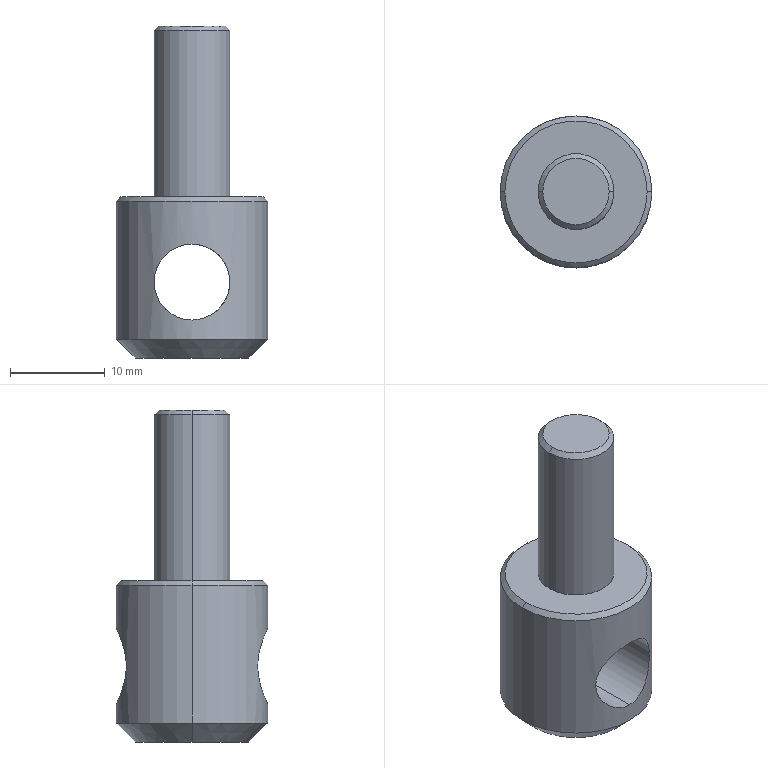Part | NX | features BREP 1 | 1 solid | 15 faces | box 16 x 16 x 35 mm | volume 3443 mm3 | cone 6 | cylinder 6 | plane 3 | commonest cylinder face diameters 8 x4 16 x2
STEP:
#1=CARTESIAN_POINT('',(-1.629,-43.754,35.));
#2=VERTEX_POINT('',#1);
#3=CARTESIAN_POINT('',(-8.629,-43.754,35.));
#4=VERTEX_POINT('',#3);
#5=CARTESIAN_POINT('',(-5.129,-43.754,35.));
#6=DIRECTION('',(0.,0.,1.));
#7=DIRECTION('',(1.,0.,0.));
#8=AXIS2_PLACEMENT_3D('',#5,#6,#7);
#9=CIRCLE('',#8,3.5);
#10=EDGE_CURVE('',#2,#4,#9,.T.);
#11=ORIENTED_EDGE('',*,*,#10,.F.);
#12=CARTESIAN_POINT('',(-1.129,-43.754,34.5));
#13=VERTEX_POINT('',#12);
#14=CARTESIAN_POINT('',(-1.629,-43.754,35.));
#15=DIRECTION('',(0.7071,0.,-0.7071));
#16=VECTOR('',#15,1000.);
#17=LINE('',#14,#16);
#18=EDGE_CURVE('',#2,#13,#17,.T.);
#19=ORIENTED_EDGE('',*,*,#18,.T.);
#20=CARTESIAN_POINT('',(-9.129,-43.754,34.5));
#21=VERTEX_POINT('',#20);
#22=CARTESIAN_POINT('',(-5.129,-43.754,34.5));
#23=DIRECTION('',(0.,0.,-1.));
#24=DIRECTION('',(1.,0.,0.));
#25=AXIS2_PLACEMENT_3D('',#22,#23,#24);
#26=CIRCLE('',#25,4.);
#27=EDGE_CURVE('',#21,#13,#26,.T.);
#28=ORIENTED_EDGE('',*,*,#27,.F.);
#29=CARTESIAN_POINT('',(-8.629,-43.754,35.));
#30=DIRECTION('',(-0.7071,0.,-0.7071));
#31=VECTOR('',#30,1000.);
#32=LINE('',#29,#31);
#33=EDGE_CURVE('',#4,#21,#32,.T.);
#34=ORIENTED_EDGE('',*,*,#33,.F.);
#35=EDGE_LOOP('',(#11,#19,#28,#34));
#36=FACE_BOUND('',#35,.T.);
#37=CARTESIAN_POINT('',(-5.129,-43.754,35.));
#38=DIRECTION('',(0.,0.,-1.));
#39=DIRECTION('',(-1.,0.,0.));
#40=AXIS2_PLACEMENT_3D('',#37,#38,#39);
#41=CONICAL_SURFACE('',#40,3.5,0.7854);
#42=ADVANCED_FACE('',(#36),#41,.T.);
#43=CARTESIAN_POINT('',(2.371,-43.754,17.));
#44=VERTEX_POINT('',#43);
#45=CARTESIAN_POINT('',(-12.629,-43.754,17.));
#46=VERTEX_POINT('',#45);
#47=CARTESIAN_POINT('',(-5.129,-43.754,17.));
#48=DIRECTION('',(0.,0.,1.));
#49=DIRECTION('',(1.,0.,0.));
#50=AXIS2_PLACEMENT_3D('',#47,#48,#49);
#51=CIRCLE('',#50,7.5);
#52=EDGE_CURVE('',#44,#46,#51,.T.);
#53=ORIENTED_EDGE('',*,*,#52,.F.);
#54=CARTESIAN_POINT('',(2.871,-43.754,16.5));
#55=VERTEX_POINT('',#54);
#56=CARTESIAN_POINT('',(2.371,-43.754,17.));
#57=DIRECTION('',(0.7071,0.,-0.7071));
#58=VECTOR('',#57,1000.);
#59=LINE('',#56,#58);
#60=EDGE_CURVE('',#44,#55,#59,.T.);
#61=ORIENTED_EDGE('',*,*,#60,.T.);
#62=CARTESIAN_POINT('',(-13.129,-43.754,16.5));
#63=VERTEX_POINT('',#62);
#64=CARTESIAN_POINT('',(-5.129,-43.754,16.5));
#65=DIRECTION('',(0.,0.,-1.));
#66=DIRECTION('',(1.,0.,0.));
#67=AXIS2_PLACEMENT_3D('',#64,#65,#66);
#68=CIRCLE('',#67,8.);
#69=EDGE_CURVE('',#63,#55,#68,.T.);
#70=ORIENTED_EDGE('',*,*,#69,.F.);
#71=CARTESIAN_POINT('',(-12.629,-43.754,17.));
#72=DIRECTION('',(-0.7071,0.,-0.7071));
#73=VECTOR('',#72,1000.);
#74=LINE('',#71,#73);
#75=EDGE_CURVE('',#46,#63,#74,.T.);
#76=ORIENTED_EDGE('',*,*,#75,.F.);
#77=EDGE_LOOP('',(#53,#61,#70,#76));
#78=FACE_BOUND('',#77,.T.);
#79=CARTESIAN_POINT('',(-5.129,-43.754,17.));
#80=DIRECTION('',(0.,0.,-1.));
#81=DIRECTION('',(-1.,0.,0.));
#82=AXIS2_PLACEMENT_3D('',#79,#80,#81);
#83=CONICAL_SURFACE('',#82,7.5,0.7854);
#84=ADVANCED_FACE('',(#78),#83,.T.);
#85=ORIENTED_EDGE('',*,*,#27,.T.);
#86=CARTESIAN_POINT('',(-1.129,-43.754,17.));
#87=VERTEX_POINT('',#86);
#88=CARTESIAN_POINT('',(-1.129,-43.754,35.));
#89=DIRECTION('',(0.,0.,-1.));
#90=VECTOR('',#89,1000.);
#91=LINE('',#88,#90);
#92=EDGE_CURVE('',#13,#87,#91,.T.);
#93=ORIENTED_EDGE('',*,*,#92,.T.);
#94=CARTESIAN_POINT('',(-9.129,-43.754,17.));
#95=VERTEX_POINT('',#94);
#96=CARTESIAN_POINT('',(-5.129,-43.754,17.));
#97=DIRECTION('',(0.,0.,1.));
#98=DIRECTION('',(1.,0.,0.));
#99=AXIS2_PLACEMENT_3D('',#96,#97,#98);
#100=CIRCLE('',#99,4.);
#101=EDGE_CURVE('',#87,#95,#100,.T.);
#102=ORIENTED_EDGE('',*,*,#101,.T.);
#103=CARTESIAN_POINT('',(-9.129,-43.754,35.));
#104=DIRECTION('',(0.,0.,-1.));
#105=VECTOR('',#104,1000.);
#106=LINE('',#103,#105);
#107=EDGE_CURVE('',#21,#95,#106,.T.);
#108=ORIENTED_EDGE('',*,*,#107,.F.);
#109=EDGE_LOOP('',(#85,#93,#102,#108));
#110=FACE_BOUND('',#109,.T.);
#111=CARTESIAN_POINT('',(-5.129,-43.754,35.));
#112=DIRECTION('',(0.,0.,-1.));
#113=DIRECTION('',(-1.,0.,0.));
#114=AXIS2_PLACEMENT_3D('',#111,#112,#113);
#115=CYLINDRICAL_SURFACE('',#114,4.);
#116=ADVANCED_FACE('',(#110),#115,.T.);
#117=CARTESIAN_POINT('',(-11.129,-43.754,0.));
#118=VERTEX_POINT('',#117);
#119=CARTESIAN_POINT('',(0.871,-43.754,0.));
#120=VERTEX_POINT('',#119);
#121=CARTESIAN_POINT('',(-5.129,-43.754,0.));
#122=DIRECTION('',(0.,0.,-1.));
#123=DIRECTION('',(1.,0.,0.));
#124=AXIS2_PLACEMENT_3D('',#121,#122,#123);
#125=CIRCLE('',#124,6.);
#126=EDGE_CURVE('',#118,#120,#125,.T.);
#127=ORIENTED_EDGE('',*,*,#126,.F.);
#128=CARTESIAN_POINT('',(-13.129,-43.754,2.));
#129=VERTEX_POINT('',#128);
#130=CARTESIAN_POINT('',(-13.129,-43.754,2.));
#131=DIRECTION('',(-0.7071,0.,0.7071));
#132=VECTOR('',#131,1000.);
#133=LINE('',#130,#132);
#134=EDGE_CURVE('',#129,#118,#133,.F.);
#135=ORIENTED_EDGE('',*,*,#134,.F.);
#136=CARTESIAN_POINT('',(2.871,-43.754,2.));
#137=VERTEX_POINT('',#136);
#138=CARTESIAN_POINT('',(-5.129,-43.754,2.));
#139=DIRECTION('',(0.,0.,1.));
#140=DIRECTION('',(1.,0.,0.));
#141=AXIS2_PLACEMENT_3D('',#138,#139,#140);
#142=CIRCLE('',#141,8.);
#143=EDGE_CURVE('',#137,#129,#142,.T.);
#144=ORIENTED_EDGE('',*,*,#143,.F.);
#145=CARTESIAN_POINT('',(2.871,-43.754,2.));
#146=DIRECTION('',(0.7071,0.,0.7071));
#147=VECTOR('',#146,1000.);
#148=LINE('',#145,#147);
#149=EDGE_CURVE('',#137,#120,#148,.F.);
#150=ORIENTED_EDGE('',*,*,#149,.T.);
#151=EDGE_LOOP('',(#127,#135,#144,#150));
#152=FACE_BOUND('',#151,.T.);
#153=CARTESIAN_POINT('',(-5.129,-43.754,2.));
#154=DIRECTION('',(0.,0.,1.));
#155=DIRECTION('',(1.,0.,0.));
#156=AXIS2_PLACEMENT_3D('',#153,#154,#155);
#157=CONICAL_SURFACE('',#156,8.,0.7854);
#158=ADVANCED_FACE('',(#152),#157,.T.);
#159=CARTESIAN_POINT('',(-5.129,-35.754,4.));
#160=VERTEX_POINT('',#159);
#161=CARTESIAN_POINT('',(-5.129,-35.754,12.));
#162=VERTEX_POINT('',#161);
#163=CARTESIAN_POINT('',(-5.129,-35.754,4.));
#164=CARTESIAN_POINT('',(-5.382,-35.754,4.));
#165=CARTESIAN_POINT('',(-5.888,-35.776,4.042));
#166=CARTESIAN_POINT('',(-6.584,-35.881,4.26));
#167=CARTESIAN_POINT('',(-7.004,-35.974,4.459));
#168=CARTESIAN_POINT('',(-7.389,-36.077,4.692));
#169=CARTESIAN_POINT('',(-7.623,-36.151,4.868));
#170=CARTESIAN_POINT('',(-7.953,-36.265,5.147));
#171=CARTESIAN_POINT('',(-8.331,-36.42,5.593));
#172=CARTESIAN_POINT('',(-8.423,-36.463,5.723));
#173=CARTESIAN_POINT('',(-8.683,-36.585,6.146));
#174=CARTESIAN_POINT('',(-8.864,-36.678,6.541));
#175=CARTESIAN_POINT('',(-9.082,-36.797,7.212));
#176=CARTESIAN_POINT('',(-9.153,-36.84,7.994));
#177=CARTESIAN_POINT('',(-9.082,-36.797,8.79));
#178=CARTESIAN_POINT('',(-8.864,-36.679,9.458));
#179=CARTESIAN_POINT('',(-8.683,-36.585,9.855));
#180=CARTESIAN_POINT('',(-8.421,-36.462,10.28));
#181=CARTESIAN_POINT('',(-8.331,-36.42,10.408));
#182=CARTESIAN_POINT('',(-7.949,-36.263,10.857));
#183=CARTESIAN_POINT('',(-7.621,-36.151,11.133));
#184=CARTESIAN_POINT('',(-7.386,-36.076,11.31));
#185=CARTESIAN_POINT('',(-7.002,-35.973,11.542));
#186=CARTESIAN_POINT('',(-6.581,-35.881,11.741));
#187=CARTESIAN_POINT('',(-5.887,-35.776,11.958));
#188=CARTESIAN_POINT('',(-5.381,-35.754,12.));
#189=CARTESIAN_POINT('',(-5.129,-35.754,12.));
#190=B_SPLINE_CURVE_WITH_KNOTS('',3,(#163,#164,#165,#166,#167,#168,#169,#170,#171,#172,#173,#174,#175,#176,#177,#178,#179,#180,#181,#182,#183,#184,#185,#186,#187,#188,#189),.UNSPECIFIED.,.F.,.F.,(4,1,1,1,1,1,1,1,1,1,1,1,1,1,1,1,1,1,1,1,1,1,1,1,4),(0.,0.0625,0.125,0.1562,0.1875,0.2188,0.25,0.2812,0.3125,0.3438,0.375,0.4375,0.5,0.5625,0.625,0.6562,0.6875,0.7188,0.75,0.7812,0.8125,0.8438,0.875,0.9375,1.),.UNSPECIFIED.);
#191=EDGE_CURVE('',#160,#162,#190,.T.);
#192=ORIENTED_EDGE('',*,*,#191,.T.);
#193=CARTESIAN_POINT('',(-5.129,-51.754,12.));
#194=VERTEX_POINT('',#193);
#195=CARTESIAN_POINT('',(-5.129,20.,12.));
#196=DIRECTION('',(0.,-1.,0.));
#197=VECTOR('',#196,1000.);
#198=LINE('',#195,#197);
#199=EDGE_CURVE('',#162,#194,#198,.T.);
#200=ORIENTED_EDGE('',*,*,#199,.T.);
#201=CARTESIAN_POINT('',(-5.129,-51.754,4.));
#202=VERTEX_POINT('',#201);
#203=CARTESIAN_POINT('',(-5.129,-51.754,12.));
#204=CARTESIAN_POINT('',(-5.382,-51.754,12.));
#205=CARTESIAN_POINT('',(-5.888,-51.731,11.958));
#206=CARTESIAN_POINT('',(-6.583,-51.626,11.74));
#207=CARTESIAN_POINT('',(-7.004,-51.534,11.541));
#208=CARTESIAN_POINT('',(-7.389,-51.43,11.308));
#209=CARTESIAN_POINT('',(-7.623,-51.356,11.132));
#210=CARTESIAN_POINT('',(-7.954,-51.242,10.852));
#211=CARTESIAN_POINT('',(-8.33,-51.088,10.409));
#212=CARTESIAN_POINT('',(-8.421,-51.045,10.279));
#213=CARTESIAN_POINT('',(-8.683,-50.923,9.855));
#214=CARTESIAN_POINT('',(-8.865,-50.829,9.457));
#215=CARTESIAN_POINT('',(-9.08,-50.711,8.796));
#216=CARTESIAN_POINT('',(-9.153,-50.668,8.005));
#217=CARTESIAN_POINT('',(-9.082,-50.71,7.212));
#218=CARTESIAN_POINT('',(-8.866,-50.828,6.547));
#219=CARTESIAN_POINT('',(-8.684,-50.922,6.148));
#220=CARTESIAN_POINT('',(-8.422,-51.045,5.722));
#221=CARTESIAN_POINT('',(-8.331,-51.087,5.593));
#222=CARTESIAN_POINT('',(-7.951,-51.243,5.146));
#223=CARTESIAN_POINT('',(-7.624,-51.356,4.869));
#224=CARTESIAN_POINT('',(-7.391,-51.43,4.694));
#225=CARTESIAN_POINT('',(-7.005,-51.533,4.459));
#226=CARTESIAN_POINT('',(-6.584,-51.626,4.26));
#227=CARTESIAN_POINT('',(-5.889,-51.731,4.042));
#228=CARTESIAN_POINT('',(-5.382,-51.754,4.));
#229=CARTESIAN_POINT('',(-5.129,-51.754,4.));
#230=B_SPLINE_CURVE_WITH_KNOTS('',3,(#203,#204,#205,#206,#207,#208,#209,#210,#211,#212,#213,#214,#215,#216,#217,#218,#219,#220,#221,#222,#223,#224,#225,#226,#227,#228,#229),.UNSPECIFIED.,.F.,.F.,(4,1,1,1,1,1,1,1,1,1,1,1,1,1,1,1,1,1,1,1,1,1,1,1,4),(0.,0.0625,0.125,0.1562,0.1875,0.2188,0.25,0.2812,0.3125,0.3438,0.375,0.4375,0.5,0.5625,0.625,0.6562,0.6875,0.7188,0.75,0.7812,0.8125,0.8438,0.875,0.9375,1.),.UNSPECIFIED.);
#231=EDGE_CURVE('',#194,#202,#230,.T.);
#232=ORIENTED_EDGE('',*,*,#231,.T.);
#233=CARTESIAN_POINT('',(-5.129,20.,4.));
#234=DIRECTION('',(0.,-1.,0.));
#235=VECTOR('',#234,1000.);
#236=LINE('',#233,#235);
#237=EDGE_CURVE('',#160,#202,#236,.T.);
#238=ORIENTED_EDGE('',*,*,#237,.F.);
#239=EDGE_LOOP('',(#192,#200,#232,#238));
#240=FACE_BOUND('',#239,.T.);
#241=CARTESIAN_POINT('',(-5.129,20.,8.));
#242=DIRECTION('',(0.,-1.,0.));
#243=DIRECTION('',(0.,0.,-1.));
#244=AXIS2_PLACEMENT_3D('',#241,#242,#243);
#245=CYLINDRICAL_SURFACE('',#244,4.);
#246=ADVANCED_FACE('',(#240),#245,.F.);
#247=ORIENTED_EDGE('',*,*,#69,.T.);
#248=CARTESIAN_POINT('',(2.871,-43.754,17.));
#249=DIRECTION('',(0.,0.,-1.));
#250=VECTOR('',#249,1000.);
#251=LINE('',#248,#250);
#252=EDGE_CURVE('',#55,#137,#251,.T.);
#253=ORIENTED_EDGE('',*,*,#252,.T.);
#254=ORIENTED_EDGE('',*,*,#143,.T.);
#255=CARTESIAN_POINT('',(-13.129,-43.754,17.));
#256=DIRECTION('',(0.,0.,-1.));
#257=VECTOR('',#256,1000.);
#258=LINE('',#255,#257);
#259=EDGE_CURVE('',#63,#129,#258,.T.);
#260=ORIENTED_EDGE('',*,*,#259,.F.);
#261=EDGE_LOOP('',(#247,#253,#254,#260));
#262=FACE_BOUND('',#261,.T.);
#263=ORIENTED_EDGE('',*,*,#191,.F.);
#264=CARTESIAN_POINT('',(-5.129,-35.754,4.));
#265=CARTESIAN_POINT('',(-4.06,-35.754,4.));
#266=CARTESIAN_POINT('',(-2.001,-36.253,4.868));
#267=CARTESIAN_POINT('',(-0.6936,-37.112,8.008));
#268=CARTESIAN_POINT('',(-1.998,-36.254,11.125));
#269=CARTESIAN_POINT('',(-4.061,-35.754,12.));
#270=CARTESIAN_POINT('',(-5.129,-35.754,12.));
#271=B_SPLINE_CURVE_WITH_KNOTS('',3,(#264,#265,#266,#267,#268,#269,#270),.UNSPECIFIED.,.F.,.F.,(4,1,1,1,4),(0.,0.25,0.5,0.75,1.),.UNSPECIFIED.);
#272=EDGE_CURVE('',#162,#160,#271,.F.);
#273=ORIENTED_EDGE('',*,*,#272,.F.);
#274=EDGE_LOOP('',(#263,#273));
#275=FACE_BOUND('',#274,.T.);
#276=CARTESIAN_POINT('',(-5.129,-43.754,17.));
#277=DIRECTION('',(0.,0.,-1.));
#278=DIRECTION('',(-1.,0.,0.));
#279=AXIS2_PLACEMENT_3D('',#276,#277,#278);
#280=CYLINDRICAL_SURFACE('',#279,8.);
#281=ADVANCED_FACE('',(#262,#275),#280,.T.);
#282=CARTESIAN_POINT('',(-5.129,-43.754,17.));
#283=DIRECTION('',(0.,0.,1.));
#284=DIRECTION('',(1.,0.,0.));
#285=AXIS2_PLACEMENT_3D('',#282,#283,#284);
#286=CIRCLE('',#285,7.5);
#287=EDGE_CURVE('',#46,#44,#286,.T.);
#288=ORIENTED_EDGE('',*,*,#287,.T.);
#289=ORIENTED_EDGE('',*,*,#52,.T.);
#290=EDGE_LOOP('',(#288,#289));
#291=FACE_BOUND('',#290,.T.);
#292=CARTESIAN_POINT('',(-5.129,-43.754,17.));
#293=DIRECTION('',(0.,0.,1.));
#294=DIRECTION('',(1.,0.,0.));
#295=AXIS2_PLACEMENT_3D('',#292,#293,#294);
#296=CIRCLE('',#295,4.);
#297=EDGE_CURVE('',#95,#87,#296,.T.);
#298=ORIENTED_EDGE('',*,*,#297,.F.);
#299=ORIENTED_EDGE('',*,*,#101,.F.);
#300=EDGE_LOOP('',(#298,#299));
#301=FACE_BOUND('',#300,.T.);
#302=CARTESIAN_POINT('',(-5.129,-43.754,17.));
#303=DIRECTION('',(0.,0.,1.));
#304=DIRECTION('',(1.,0.,0.));
#305=AXIS2_PLACEMENT_3D('',#302,#303,#304);
#306=PLANE('',#305);
#307=ADVANCED_FACE('',(#291,#301),#306,.T.);
#308=ORIENTED_EDGE('',*,*,#252,.F.);
#309=CARTESIAN_POINT('',(-5.129,-43.754,16.5));
#310=DIRECTION('',(0.,0.,-1.));
#311=DIRECTION('',(1.,0.,0.));
#312=AXIS2_PLACEMENT_3D('',#309,#310,#311);
#313=CIRCLE('',#312,8.);
#314=EDGE_CURVE('',#55,#63,#313,.T.);
#315=ORIENTED_EDGE('',*,*,#314,.T.);
#316=ORIENTED_EDGE('',*,*,#259,.T.);
#317=CARTESIAN_POINT('',(-5.129,-43.754,2.));
#318=DIRECTION('',(0.,0.,1.));
#319=DIRECTION('',(1.,0.,0.));
#320=AXIS2_PLACEMENT_3D('',#317,#318,#319);
#321=CIRCLE('',#320,8.);
#322=EDGE_CURVE('',#129,#137,#321,.T.);
#323=ORIENTED_EDGE('',*,*,#322,.T.);
#324=EDGE_LOOP('',(#308,#315,#316,#323));
#325=FACE_BOUND('',#324,.T.);
#326=CARTESIAN_POINT('',(-5.129,-51.754,12.));
#327=CARTESIAN_POINT('',(-4.063,-51.754,12.));
#328=CARTESIAN_POINT('',(-2.004,-51.256,11.136));
#329=CARTESIAN_POINT('',(-0.6923,-50.395,7.992));
#330=CARTESIAN_POINT('',(-2.,-51.254,4.873));
#331=CARTESIAN_POINT('',(-4.06,-51.754,4.));
#332=CARTESIAN_POINT('',(-5.129,-51.754,4.));
#333=B_SPLINE_CURVE_WITH_KNOTS('',3,(#326,#327,#328,#329,#330,#331,#332),.UNSPECIFIED.,.F.,.F.,(4,1,1,1,4),(0.,0.25,0.5,0.75,1.),.UNSPECIFIED.);
#334=EDGE_CURVE('',#202,#194,#333,.F.);
#335=ORIENTED_EDGE('',*,*,#334,.F.);
#336=ORIENTED_EDGE('',*,*,#231,.F.);
#337=EDGE_LOOP('',(#335,#336));
#338=FACE_BOUND('',#337,.T.);
#339=CARTESIAN_POINT('',(-5.129,-43.754,17.));
#340=DIRECTION('',(0.,0.,-1.));
#341=DIRECTION('',(-1.,0.,0.));
#342=AXIS2_PLACEMENT_3D('',#339,#340,#341);
#343=CYLINDRICAL_SURFACE('',#342,8.);
#344=ADVANCED_FACE('',(#325,#338),#343,.T.);
#345=CARTESIAN_POINT('',(-5.129,-43.754,0.));
#346=DIRECTION('',(0.,0.,-1.));
#347=DIRECTION('',(1.,0.,0.));
#348=AXIS2_PLACEMENT_3D('',#345,#346,#347);
#349=CIRCLE('',#348,6.);
#350=EDGE_CURVE('',#120,#118,#349,.T.);
#351=ORIENTED_EDGE('',*,*,#350,.T.);
#352=ORIENTED_EDGE('',*,*,#126,.T.);
#353=EDGE_LOOP('',(#351,#352));
#354=FACE_BOUND('',#353,.T.);
#355=CARTESIAN_POINT('',(-5.129,-43.754,0.));
#356=DIRECTION('',(0.,0.,1.));
#357=DIRECTION('',(1.,0.,0.));
#358=AXIS2_PLACEMENT_3D('',#355,#356,#357);
#359=PLANE('',#358);
#360=ADVANCED_FACE('',(#354),#359,.F.);
#361=ORIENTED_EDGE('',*,*,#199,.F.);
#362=ORIENTED_EDGE('',*,*,#272,.T.);
#363=ORIENTED_EDGE('',*,*,#237,.T.);
#364=ORIENTED_EDGE('',*,*,#334,.T.);
#365=EDGE_LOOP('',(#361,#362,#363,#364));
#366=FACE_BOUND('',#365,.T.);
#367=CARTESIAN_POINT('',(-5.129,20.,8.));
#368=DIRECTION('',(0.,-1.,0.));
#369=DIRECTION('',(0.,0.,-1.));
#370=AXIS2_PLACEMENT_3D('',#367,#368,#369);
#371=CYLINDRICAL_SURFACE('',#370,4.);
#372=ADVANCED_FACE('',(#366),#371,.F.);
#373=ORIENTED_EDGE('',*,*,#134,.T.);
#374=ORIENTED_EDGE('',*,*,#350,.F.);
#375=ORIENTED_EDGE('',*,*,#149,.F.);
#376=ORIENTED_EDGE('',*,*,#322,.F.);
#377=EDGE_LOOP('',(#373,#374,#375,#376));
#378=FACE_BOUND('',#377,.T.);
#379=CARTESIAN_POINT('',(-5.129,-43.754,2.));
#380=DIRECTION('',(0.,0.,1.));
#381=DIRECTION('',(1.,0.,0.));
#382=AXIS2_PLACEMENT_3D('',#379,#380,#381);
#383=CONICAL_SURFACE('',#382,8.,0.7854);
#384=ADVANCED_FACE('',(#378),#383,.T.);
#385=ORIENTED_EDGE('',*,*,#92,.F.);
#386=CARTESIAN_POINT('',(-5.129,-43.754,34.5));
#387=DIRECTION('',(0.,0.,-1.));
#388=DIRECTION('',(1.,0.,0.));
#389=AXIS2_PLACEMENT_3D('',#386,#387,#388);
#390=CIRCLE('',#389,4.);
#391=EDGE_CURVE('',#13,#21,#390,.T.);
#392=ORIENTED_EDGE('',*,*,#391,.T.);
#393=ORIENTED_EDGE('',*,*,#107,.T.);
#394=ORIENTED_EDGE('',*,*,#297,.T.);
#395=EDGE_LOOP('',(#385,#392,#393,#394));
#396=FACE_BOUND('',#395,.T.);
#397=CARTESIAN_POINT('',(-5.129,-43.754,35.));
#398=DIRECTION('',(0.,0.,-1.));
#399=DIRECTION('',(-1.,0.,0.));
#400=AXIS2_PLACEMENT_3D('',#397,#398,#399);
#401=CYLINDRICAL_SURFACE('',#400,4.);
#402=ADVANCED_FACE('',(#396),#401,.T.);
#403=CARTESIAN_POINT('',(-5.129,-43.754,35.));
#404=DIRECTION('',(0.,0.,1.));
#405=DIRECTION('',(1.,0.,0.));
#406=AXIS2_PLACEMENT_3D('',#403,#404,#405);
#407=CIRCLE('',#406,3.5);
#408=EDGE_CURVE('',#4,#2,#407,.T.);
#409=ORIENTED_EDGE('',*,*,#408,.T.);
#410=ORIENTED_EDGE('',*,*,#10,.T.);
#411=EDGE_LOOP('',(#409,#410));
#412=FACE_BOUND('',#411,.T.);
#413=CARTESIAN_POINT('',(-5.129,-43.754,35.));
#414=DIRECTION('',(0.,0.,1.));
#415=DIRECTION('',(1.,0.,0.));
#416=AXIS2_PLACEMENT_3D('',#413,#414,#415);
#417=PLANE('',#416);
#418=ADVANCED_FACE('',(#412),#417,.T.);
#419=ORIENTED_EDGE('',*,*,#60,.F.);
#420=ORIENTED_EDGE('',*,*,#287,.F.);
#421=ORIENTED_EDGE('',*,*,#75,.T.);
#422=ORIENTED_EDGE('',*,*,#314,.F.);
#423=EDGE_LOOP('',(#419,#420,#421,#422));
#424=FACE_BOUND('',#423,.T.);
#425=CARTESIAN_POINT('',(-5.129,-43.754,17.));
#426=DIRECTION('',(0.,0.,-1.));
#427=DIRECTION('',(-1.,0.,0.));
#428=AXIS2_PLACEMENT_3D('',#425,#426,#427);
#429=CONICAL_SURFACE('',#428,7.5,0.7854);
#430=ADVANCED_FACE('',(#424),#429,.T.);
#431=ORIENTED_EDGE('',*,*,#18,.F.);
#432=ORIENTED_EDGE('',*,*,#408,.F.);
#433=ORIENTED_EDGE('',*,*,#33,.T.);
#434=ORIENTED_EDGE('',*,*,#391,.F.);
#435=EDGE_LOOP('',(#431,#432,#433,#434));
#436=FACE_BOUND('',#435,.T.);
#437=CARTESIAN_POINT('',(-5.129,-43.754,35.));
#438=DIRECTION('',(0.,0.,-1.));
#439=DIRECTION('',(-1.,0.,0.));
#440=AXIS2_PLACEMENT_3D('',#437,#438,#439);
#441=CONICAL_SURFACE('',#440,3.5,0.7854);
#442=ADVANCED_FACE('',(#436),#441,.T.);
#443=CLOSED_SHELL('',(#42,#84,#116,#158,#246,#281,#307,#344,#360,#372,#384,#402,#418,#430,#442));
#444=MANIFOLD_SOLID_BREP('',#443);
#445=(LENGTH_UNIT()NAMED_UNIT(*)SI_UNIT(.MILLI.,.METRE.));
#446=UNCERTAINTY_MEASURE_WITH_UNIT(LENGTH_MEASURE(0.0508),#445,'','');
#447=(NAMED_UNIT(*)PLANE_ANGLE_UNIT()SI_UNIT($,.RADIAN.));
#448=(NAMED_UNIT(*)SI_UNIT($,.STERADIAN.)SOLID_ANGLE_UNIT());
#449=(GEOMETRIC_REPRESENTATION_CONTEXT(3)GLOBAL_UNCERTAINTY_ASSIGNED_CONTEXT((#446))GLOBAL_UNIT_ASSIGNED_CONTEXT((#445,#447,#448))REPRESENTATION_CONTEXT('',''));
#450=ADVANCED_BREP_SHAPE_REPRESENTATION('',(#444),#449);